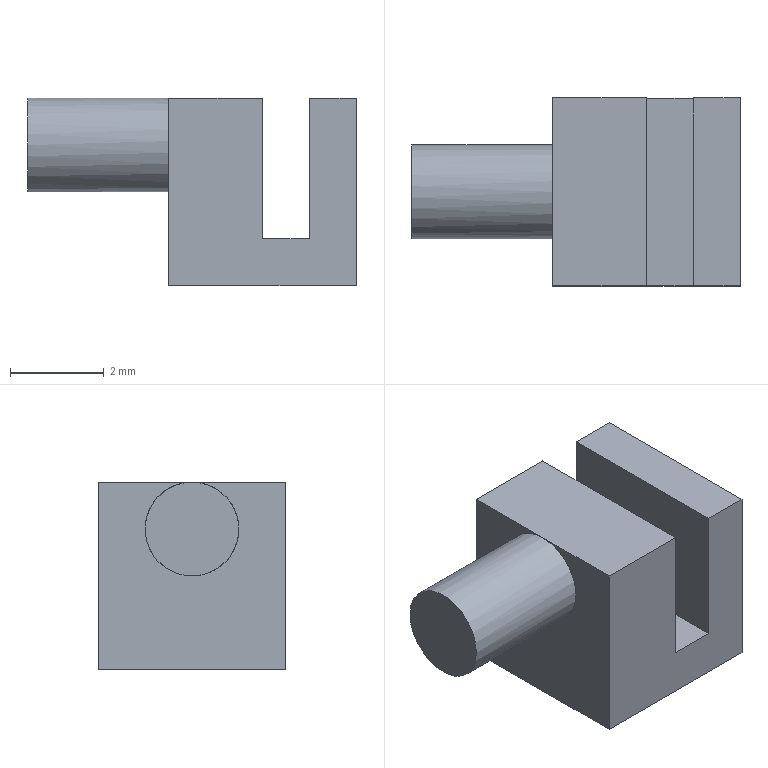Part | STEP file | 1-63.6 | 1 solid | 12 faces | box 7 x 4 x 4 mm | volume 61.425 mm3 | plane 11 | cylinder 1 | commonest cylinder face diameters 2 x1
STEP:
#1=CARTESIAN_POINT('',(0.,0.,0.));
#2=DIRECTION('',(0.,0.,1.));
#3=DIRECTION('',(1.,0.,0.));
#4=AXIS2_PLACEMENT_3D('',#1,#2,#3);
#5=CARTESIAN_POINT('',(-1.5,1.,0.));
#6=VERTEX_POINT('',#5);
#7=CARTESIAN_POINT('',(-1.5,0.,0.));
#8=DIRECTION('',(1.,0.,0.));
#9=DIRECTION('',(0.,1.,0.));
#10=AXIS2_PLACEMENT_3D('',#7,#8,#9);
#11=CIRCLE('',#10,1.);
#12=CARTESIAN_POINT('',(-1.5,-0.2679,0.));
#13=DIRECTION('',(1.,0.,0.));
#14=DIRECTION('',(0.,1.,0.));
#15=AXIS2_PLACEMENT_3D('',#12,#13,#14);
#16=PLANE('',#15);
#17=CARTESIAN_POINT('',(0.2679,0.));
#18=DIRECTION('',(1.,0.));
#19=AXIS2_PLACEMENT_2D('',#17,#18);
#20=CIRCLE('',#19,1.);
#21=(GEOMETRIC_REPRESENTATION_CONTEXT(2)PARAMETRIC_REPRESENTATION_CONTEXT()REPRESENTATION_CONTEXT('',''));
#22=DEFINITIONAL_REPRESENTATION('',(#20),#21);
#23=PCURVE('',#16,#22);
#24=CARTESIAN_POINT('',(1.5,0.,0.));
#25=DIRECTION('',(-1.,0.,0.));
#26=DIRECTION('',(0.,1.,0.));
#27=AXIS2_PLACEMENT_3D('',#24,#25,#26);
#28=CYLINDRICAL_SURFACE('',#27,1.);
#29=CARTESIAN_POINT('',(6.283,3.));
#30=DIRECTION('',(-1.,0.));
#31=VECTOR('',#30,1.);
#32=LINE('',#29,#31);
#33=(GEOMETRIC_REPRESENTATION_CONTEXT(2)PARAMETRIC_REPRESENTATION_CONTEXT()REPRESENTATION_CONTEXT('',''));
#34=DEFINITIONAL_REPRESENTATION('',(#32),#33);
#35=PCURVE('',#28,#34);
#36=SURFACE_CURVE('',#11,(#23,#35),.PCURVE_S1.);
#37=EDGE_CURVE('',#6,#6,#36,.T.);
#38=ORIENTED_EDGE('',*,*,#37,.T.);
#39=EDGE_LOOP('',(#38));
#40=FACE_BOUND('',#39,.F.);
#41=ADVANCED_FACE('',(#40),#16,.F.);
#42=CARTESIAN_POINT('',(1.5,1.,0.));
#43=VERTEX_POINT('',#42);
#44=CARTESIAN_POINT('',(1.5,1.,0.));
#45=DIRECTION('',(-1.,0.,0.));
#46=VECTOR('',#45,1.);
#47=LINE('',#44,#46);
#48=CARTESIAN_POINT('',(6.283,0.));
#49=DIRECTION('',(0.,1.));
#50=VECTOR('',#49,1.);
#51=LINE('',#48,#50);
#52=(GEOMETRIC_REPRESENTATION_CONTEXT(2)PARAMETRIC_REPRESENTATION_CONTEXT()REPRESENTATION_CONTEXT('',''));
#53=DEFINITIONAL_REPRESENTATION('',(#51),#52);
#54=PCURVE('',#28,#53);
#55=CARTESIAN_POINT('',(0.,0.));
#56=DIRECTION('',(0.,1.));
#57=VECTOR('',#56,1.);
#58=LINE('',#55,#57);
#59=(GEOMETRIC_REPRESENTATION_CONTEXT(2)PARAMETRIC_REPRESENTATION_CONTEXT()REPRESENTATION_CONTEXT('',''));
#60=DEFINITIONAL_REPRESENTATION('',(#58),#59);
#61=PCURVE('',#28,#60);
#62=SEAM_CURVE('',#47,(#54,#61),.PCURVE_S1.);
#63=EDGE_CURVE('',#43,#6,#62,.T.);
#64=ORIENTED_EDGE('',*,*,#63,.T.);
#65=ORIENTED_EDGE('',*,*,#37,.T.);
#66=ORIENTED_EDGE('',*,*,#63,.F.);
#67=CARTESIAN_POINT('',(1.5,0.,1.));
#68=VERTEX_POINT('',#67);
#69=CARTESIAN_POINT('',(1.5,0.,0.));
#70=DIRECTION('',(1.,0.,0.));
#71=DIRECTION('',(0.,0.,1.));
#72=AXIS2_PLACEMENT_3D('',#69,#70,#71);
#73=CIRCLE('',#72,1.);
#74=CARTESIAN_POINT('',(4.712,0.));
#75=DIRECTION('',(-1.,0.));
#76=VECTOR('',#75,1.);
#77=LINE('',#74,#76);
#78=(GEOMETRIC_REPRESENTATION_CONTEXT(2)PARAMETRIC_REPRESENTATION_CONTEXT()REPRESENTATION_CONTEXT('',''));
#79=DEFINITIONAL_REPRESENTATION('',(#77),#78);
#80=PCURVE('',#28,#79);
#81=CARTESIAN_POINT('',(1.5,0.,-1.));
#82=DIRECTION('',(1.,0.,0.));
#83=DIRECTION('',(0.,0.,-1.));
#84=AXIS2_PLACEMENT_3D('',#81,#82,#83);
#85=PLANE('',#84);
#86=CARTESIAN_POINT('',(-1.,0.));
#87=DIRECTION('',(-1.,0.));
#88=AXIS2_PLACEMENT_2D('',#86,#87);
#89=CIRCLE('',#88,1.);
#90=(GEOMETRIC_REPRESENTATION_CONTEXT(2)PARAMETRIC_REPRESENTATION_CONTEXT()REPRESENTATION_CONTEXT('',''));
#91=DEFINITIONAL_REPRESENTATION('',(#89),#90);
#92=PCURVE('',#85,#91);
#93=SURFACE_CURVE('',#73,(#80,#92),.PCURVE_S1.);
#94=EDGE_CURVE('',#68,#43,#93,.T.);
#95=ORIENTED_EDGE('',*,*,#94,.F.);
#96=CARTESIAN_POINT('',(1.5,0.,0.));
#97=DIRECTION('',(1.,0.,0.));
#98=DIRECTION('',(0.,1.,0.));
#99=AXIS2_PLACEMENT_3D('',#96,#97,#98);
#100=CIRCLE('',#99,1.);
#101=CARTESIAN_POINT('',(6.283,0.));
#102=DIRECTION('',(-1.,0.));
#103=VECTOR('',#102,1.);
#104=LINE('',#101,#103);
#105=(GEOMETRIC_REPRESENTATION_CONTEXT(2)PARAMETRIC_REPRESENTATION_CONTEXT()REPRESENTATION_CONTEXT('',''));
#106=DEFINITIONAL_REPRESENTATION('',(#104),#105);
#107=PCURVE('',#28,#106);
#108=CARTESIAN_POINT('',(-1.,0.));
#109=DIRECTION('',(0.,1.));
#110=AXIS2_PLACEMENT_2D('',#108,#109);
#111=CIRCLE('',#110,1.);
#112=(GEOMETRIC_REPRESENTATION_CONTEXT(2)PARAMETRIC_REPRESENTATION_CONTEXT()REPRESENTATION_CONTEXT('',''));
#113=DEFINITIONAL_REPRESENTATION('',(#111),#112);
#114=PCURVE('',#85,#113);
#115=SURFACE_CURVE('',#100,(#107,#114),.PCURVE_S1.);
#116=EDGE_CURVE('',#43,#68,#115,.T.);
#117=ORIENTED_EDGE('',*,*,#116,.F.);
#118=EDGE_LOOP('',(#64,#65,#66,#95,#117));
#119=FACE_BOUND('',#118,.T.);
#120=ADVANCED_FACE('',(#119),#28,.T.);
#121=CARTESIAN_POINT('',(1.5,2.,1.));
#122=VERTEX_POINT('',#121);
#123=CARTESIAN_POINT('',(1.5,0.,1.));
#124=VERTEX_POINT('',#123);
#125=CARTESIAN_POINT('',(1.5,2.,1.));
#126=DIRECTION('',(0.,-1.,0.));
#127=VECTOR('',#126,1.);
#128=LINE('',#125,#127);
#129=CARTESIAN_POINT('',(-2.,2.));
#130=DIRECTION('',(0.,-1.));
#131=VECTOR('',#130,1.);
#132=LINE('',#129,#131);
#133=(GEOMETRIC_REPRESENTATION_CONTEXT(2)PARAMETRIC_REPRESENTATION_CONTEXT()REPRESENTATION_CONTEXT('',''));
#134=DEFINITIONAL_REPRESENTATION('',(#132),#133);
#135=PCURVE('',#85,#134);
#136=CARTESIAN_POINT('',(3.5,0.,1.));
#137=DIRECTION('',(0.,0.,1.));
#138=DIRECTION('',(0.,-1.,0.));
#139=AXIS2_PLACEMENT_3D('',#136,#137,#138);
#140=PLANE('',#139);
#141=CARTESIAN_POINT('',(-2.,-2.));
#142=DIRECTION('',(1.,0.));
#143=VECTOR('',#142,1.);
#144=LINE('',#141,#143);
#145=(GEOMETRIC_REPRESENTATION_CONTEXT(2)PARAMETRIC_REPRESENTATION_CONTEXT()REPRESENTATION_CONTEXT('',''));
#146=DEFINITIONAL_REPRESENTATION('',(#144),#145);
#147=PCURVE('',#140,#146);
#148=SURFACE_CURVE('',#128,(#135,#147),.PCURVE_S1.);
#149=EDGE_CURVE('',#122,#124,#148,.T.);
#150=ORIENTED_EDGE('',*,*,#149,.T.);
#151=CARTESIAN_POINT('',(1.5,-2.,1.));
#152=VERTEX_POINT('',#151);
#153=CARTESIAN_POINT('',(1.5,0.,1.));
#154=DIRECTION('',(0.,-1.,0.));
#155=VECTOR('',#154,1.);
#156=LINE('',#153,#155);
#157=CARTESIAN_POINT('',(-2.,0.));
#158=DIRECTION('',(0.,-1.));
#159=VECTOR('',#158,1.);
#160=LINE('',#157,#159);
#161=(GEOMETRIC_REPRESENTATION_CONTEXT(2)PARAMETRIC_REPRESENTATION_CONTEXT()REPRESENTATION_CONTEXT('',''));
#162=DEFINITIONAL_REPRESENTATION('',(#160),#161);
#163=PCURVE('',#85,#162);
#164=CARTESIAN_POINT('',(0.,-2.));
#165=DIRECTION('',(1.,0.));
#166=VECTOR('',#165,1.);
#167=LINE('',#164,#166);
#168=(GEOMETRIC_REPRESENTATION_CONTEXT(2)PARAMETRIC_REPRESENTATION_CONTEXT()REPRESENTATION_CONTEXT('',''));
#169=DEFINITIONAL_REPRESENTATION('',(#167),#168);
#170=PCURVE('',#140,#169);
#171=SURFACE_CURVE('',#156,(#163,#170),.PCURVE_S1.);
#172=EDGE_CURVE('',#124,#152,#171,.T.);
#173=ORIENTED_EDGE('',*,*,#172,.T.);
#174=CARTESIAN_POINT('',(1.5,-2.,-3.));
#175=VERTEX_POINT('',#174);
#176=CARTESIAN_POINT('',(1.5,-2.,1.));
#177=DIRECTION('',(0.,0.,-1.));
#178=VECTOR('',#177,1.);
#179=LINE('',#176,#178);
#180=CARTESIAN_POINT('',(-2.,-2.));
#181=DIRECTION('',(1.,0.));
#182=VECTOR('',#181,1.);
#183=LINE('',#180,#182);
#184=(GEOMETRIC_REPRESENTATION_CONTEXT(2)PARAMETRIC_REPRESENTATION_CONTEXT()REPRESENTATION_CONTEXT('',''));
#185=DEFINITIONAL_REPRESENTATION('',(#183),#184);
#186=PCURVE('',#85,#185);
#187=CARTESIAN_POINT('',(3.5,-2.,-1.));
#188=DIRECTION('',(0.,-1.,0.));
#189=DIRECTION('',(0.,0.,-1.));
#190=AXIS2_PLACEMENT_3D('',#187,#188,#189);
#191=PLANE('',#190);
#192=CARTESIAN_POINT('',(-2.,-2.));
#193=DIRECTION('',(1.,0.));
#194=VECTOR('',#193,1.);
#195=LINE('',#192,#194);
#196=(GEOMETRIC_REPRESENTATION_CONTEXT(2)PARAMETRIC_REPRESENTATION_CONTEXT()REPRESENTATION_CONTEXT('',''));
#197=DEFINITIONAL_REPRESENTATION('',(#195),#196);
#198=PCURVE('',#191,#197);
#199=SURFACE_CURVE('',#179,(#186,#198),.PCURVE_S1.);
#200=EDGE_CURVE('',#152,#175,#199,.T.);
#201=ORIENTED_EDGE('',*,*,#200,.T.);
#202=CARTESIAN_POINT('',(1.5,2.,-3.));
#203=VERTEX_POINT('',#202);
#204=CARTESIAN_POINT('',(1.5,-2.,-3.));
#205=DIRECTION('',(0.,1.,0.));
#206=VECTOR('',#205,1.);
#207=LINE('',#204,#206);
#208=CARTESIAN_POINT('',(2.,-2.));
#209=DIRECTION('',(0.,1.));
#210=VECTOR('',#209,1.);
#211=LINE('',#208,#210);
#212=(GEOMETRIC_REPRESENTATION_CONTEXT(2)PARAMETRIC_REPRESENTATION_CONTEXT()REPRESENTATION_CONTEXT('',''));
#213=DEFINITIONAL_REPRESENTATION('',(#211),#212);
#214=PCURVE('',#85,#213);
#215=CARTESIAN_POINT('',(3.5,0.,-3.));
#216=DIRECTION('',(0.,0.,-1.));
#217=DIRECTION('',(0.,1.,0.));
#218=AXIS2_PLACEMENT_3D('',#215,#216,#217);
#219=PLANE('',#218);
#220=CARTESIAN_POINT('',(-2.,-2.));
#221=DIRECTION('',(1.,0.));
#222=VECTOR('',#221,1.);
#223=LINE('',#220,#222);
#224=(GEOMETRIC_REPRESENTATION_CONTEXT(2)PARAMETRIC_REPRESENTATION_CONTEXT()REPRESENTATION_CONTEXT('',''));
#225=DEFINITIONAL_REPRESENTATION('',(#223),#224);
#226=PCURVE('',#219,#225);
#227=SURFACE_CURVE('',#207,(#214,#226),.PCURVE_S1.);
#228=EDGE_CURVE('',#175,#203,#227,.T.);
#229=ORIENTED_EDGE('',*,*,#228,.T.);
#230=CARTESIAN_POINT('',(1.5,2.,-3.));
#231=DIRECTION('',(0.,0.,1.));
#232=VECTOR('',#231,1.);
#233=LINE('',#230,#232);
#234=CARTESIAN_POINT('',(2.,2.));
#235=DIRECTION('',(-1.,0.));
#236=VECTOR('',#235,1.);
#237=LINE('',#234,#236);
#238=(GEOMETRIC_REPRESENTATION_CONTEXT(2)PARAMETRIC_REPRESENTATION_CONTEXT()REPRESENTATION_CONTEXT('',''));
#239=DEFINITIONAL_REPRESENTATION('',(#237),#238);
#240=PCURVE('',#85,#239);
#241=CARTESIAN_POINT('',(3.5,2.,-1.));
#242=DIRECTION('',(0.,1.,0.));
#243=DIRECTION('',(0.,0.,1.));
#244=AXIS2_PLACEMENT_3D('',#241,#242,#243);
#245=PLANE('',#244);
#246=CARTESIAN_POINT('',(-2.,-2.));
#247=DIRECTION('',(1.,0.));
#248=VECTOR('',#247,1.);
#249=LINE('',#246,#248);
#250=(GEOMETRIC_REPRESENTATION_CONTEXT(2)PARAMETRIC_REPRESENTATION_CONTEXT()REPRESENTATION_CONTEXT('',''));
#251=DEFINITIONAL_REPRESENTATION('',(#249),#250);
#252=PCURVE('',#245,#251);
#253=SURFACE_CURVE('',#233,(#240,#252),.PCURVE_S1.);
#254=EDGE_CURVE('',#203,#122,#253,.T.);
#255=ORIENTED_EDGE('',*,*,#254,.T.);
#256=EDGE_LOOP('',(#150,#173,#201,#229,#255));
#257=FACE_BOUND('',#256,.F.);
#258=ORIENTED_EDGE('',*,*,#116,.F.);
#259=ORIENTED_EDGE('',*,*,#94,.F.);
#260=EDGE_LOOP('',(#258,#259));
#261=FACE_BOUND('',#260,.F.);
#262=ADVANCED_FACE('',(#257,#261),#85,.F.);
#263=ORIENTED_EDGE('',*,*,#228,.T.);
#264=CARTESIAN_POINT('',(5.5,2.,-3.));
#265=VERTEX_POINT('',#264);
#266=CARTESIAN_POINT('',(1.5,2.,-3.));
#267=DIRECTION('',(1.,0.,0.));
#268=VECTOR('',#267,1.);
#269=LINE('',#266,#268);
#270=CARTESIAN_POINT('',(2.,-2.));
#271=DIRECTION('',(0.,1.));
#272=VECTOR('',#271,1.);
#273=LINE('',#270,#272);
#274=(GEOMETRIC_REPRESENTATION_CONTEXT(2)PARAMETRIC_REPRESENTATION_CONTEXT()REPRESENTATION_CONTEXT('',''));
#275=DEFINITIONAL_REPRESENTATION('',(#273),#274);
#276=PCURVE('',#219,#275);
#277=CARTESIAN_POINT('',(-2.,-2.));
#278=DIRECTION('',(0.,1.));
#279=VECTOR('',#278,1.);
#280=LINE('',#277,#279);
#281=(GEOMETRIC_REPRESENTATION_CONTEXT(2)PARAMETRIC_REPRESENTATION_CONTEXT()REPRESENTATION_CONTEXT('',''));
#282=DEFINITIONAL_REPRESENTATION('',(#280),#281);
#283=PCURVE('',#245,#282);
#284=SURFACE_CURVE('',#269,(#276,#283),.PCURVE_S1.);
#285=EDGE_CURVE('',#203,#265,#284,.T.);
#286=ORIENTED_EDGE('',*,*,#285,.T.);
#287=CARTESIAN_POINT('',(5.5,-2.,-3.));
#288=VERTEX_POINT('',#287);
#289=CARTESIAN_POINT('',(5.5,-2.,-3.));
#290=DIRECTION('',(0.,1.,0.));
#291=VECTOR('',#290,1.);
#292=LINE('',#289,#291);
#293=CARTESIAN_POINT('',(-2.,2.));
#294=DIRECTION('',(1.,0.));
#295=VECTOR('',#294,1.);
#296=LINE('',#293,#295);
#297=(GEOMETRIC_REPRESENTATION_CONTEXT(2)PARAMETRIC_REPRESENTATION_CONTEXT()REPRESENTATION_CONTEXT('',''));
#298=DEFINITIONAL_REPRESENTATION('',(#296),#297);
#299=PCURVE('',#219,#298);
#300=CARTESIAN_POINT('',(5.5,0.,-1.));
#301=DIRECTION('',(1.,0.,0.));
#302=DIRECTION('',(0.,0.,-1.));
#303=AXIS2_PLACEMENT_3D('',#300,#301,#302);
#304=PLANE('',#303);
#305=CARTESIAN_POINT('',(2.,-2.));
#306=DIRECTION('',(0.,1.));
#307=VECTOR('',#306,1.);
#308=LINE('',#305,#307);
#309=(GEOMETRIC_REPRESENTATION_CONTEXT(2)PARAMETRIC_REPRESENTATION_CONTEXT()REPRESENTATION_CONTEXT('',''));
#310=DEFINITIONAL_REPRESENTATION('',(#308),#309);
#311=PCURVE('',#304,#310);
#312=SURFACE_CURVE('',#292,(#299,#311),.PCURVE_S1.);
#313=EDGE_CURVE('',#288,#265,#312,.T.);
#314=ORIENTED_EDGE('',*,*,#313,.F.);
#315=CARTESIAN_POINT('',(1.5,-2.,-3.));
#316=DIRECTION('',(1.,0.,0.));
#317=VECTOR('',#316,1.);
#318=LINE('',#315,#317);
#319=CARTESIAN_POINT('',(-2.,-2.));
#320=DIRECTION('',(0.,1.));
#321=VECTOR('',#320,1.);
#322=LINE('',#319,#321);
#323=(GEOMETRIC_REPRESENTATION_CONTEXT(2)PARAMETRIC_REPRESENTATION_CONTEXT()REPRESENTATION_CONTEXT('',''));
#324=DEFINITIONAL_REPRESENTATION('',(#322),#323);
#325=PCURVE('',#219,#324);
#326=CARTESIAN_POINT('',(2.,-2.));
#327=DIRECTION('',(0.,1.));
#328=VECTOR('',#327,1.);
#329=LINE('',#326,#328);
#330=(GEOMETRIC_REPRESENTATION_CONTEXT(2)PARAMETRIC_REPRESENTATION_CONTEXT()REPRESENTATION_CONTEXT('',''));
#331=DEFINITIONAL_REPRESENTATION('',(#329),#330);
#332=PCURVE('',#191,#331);
#333=SURFACE_CURVE('',#318,(#325,#332),.PCURVE_S1.);
#334=EDGE_CURVE('',#175,#288,#333,.T.);
#335=ORIENTED_EDGE('',*,*,#334,.F.);
#336=EDGE_LOOP('',(#263,#286,#314,#335));
#337=FACE_BOUND('',#336,.T.);
#338=ADVANCED_FACE('',(#337),#219,.T.);
#339=CARTESIAN_POINT('',(5.5,-2.,1.));
#340=VERTEX_POINT('',#339);
#341=CARTESIAN_POINT('',(5.5,-2.,1.));
#342=DIRECTION('',(0.,0.,-1.));
#343=VECTOR('',#342,1.);
#344=LINE('',#341,#343);
#345=CARTESIAN_POINT('',(-2.,-2.));
#346=DIRECTION('',(1.,0.));
#347=VECTOR('',#346,1.);
#348=LINE('',#345,#347);
#349=(GEOMETRIC_REPRESENTATION_CONTEXT(2)PARAMETRIC_REPRESENTATION_CONTEXT()REPRESENTATION_CONTEXT('',''));
#350=DEFINITIONAL_REPRESENTATION('',(#348),#349);
#351=PCURVE('',#304,#350);
#352=CARTESIAN_POINT('',(-2.,2.));
#353=DIRECTION('',(1.,0.));
#354=VECTOR('',#353,1.);
#355=LINE('',#352,#354);
#356=(GEOMETRIC_REPRESENTATION_CONTEXT(2)PARAMETRIC_REPRESENTATION_CONTEXT()REPRESENTATION_CONTEXT('',''));
#357=DEFINITIONAL_REPRESENTATION('',(#355),#356);
#358=PCURVE('',#191,#357);
#359=SURFACE_CURVE('',#344,(#351,#358),.PCURVE_S1.);
#360=EDGE_CURVE('',#340,#288,#359,.T.);
#361=ORIENTED_EDGE('',*,*,#360,.T.);
#362=ORIENTED_EDGE('',*,*,#313,.T.);
#363=CARTESIAN_POINT('',(5.5,2.,1.));
#364=VERTEX_POINT('',#363);
#365=CARTESIAN_POINT('',(5.5,2.,-3.));
#366=DIRECTION('',(0.,0.,1.));
#367=VECTOR('',#366,1.);
#368=LINE('',#365,#367);
#369=CARTESIAN_POINT('',(2.,2.));
#370=DIRECTION('',(-1.,0.));
#371=VECTOR('',#370,1.);
#372=LINE('',#369,#371);
#373=(GEOMETRIC_REPRESENTATION_CONTEXT(2)PARAMETRIC_REPRESENTATION_CONTEXT()REPRESENTATION_CONTEXT('',''));
#374=DEFINITIONAL_REPRESENTATION('',(#372),#373);
#375=PCURVE('',#304,#374);
#376=CARTESIAN_POINT('',(-2.,2.));
#377=DIRECTION('',(1.,0.));
#378=VECTOR('',#377,1.);
#379=LINE('',#376,#378);
#380=(GEOMETRIC_REPRESENTATION_CONTEXT(2)PARAMETRIC_REPRESENTATION_CONTEXT()REPRESENTATION_CONTEXT('',''));
#381=DEFINITIONAL_REPRESENTATION('',(#379),#380);
#382=PCURVE('',#245,#381);
#383=SURFACE_CURVE('',#368,(#375,#382),.PCURVE_S1.);
#384=EDGE_CURVE('',#265,#364,#383,.T.);
#385=ORIENTED_EDGE('',*,*,#384,.T.);
#386=CARTESIAN_POINT('',(5.5,2.,1.));
#387=DIRECTION('',(0.,-1.,0.));
#388=VECTOR('',#387,1.);
#389=LINE('',#386,#388);
#390=CARTESIAN_POINT('',(-2.,2.));
#391=DIRECTION('',(0.,-1.));
#392=VECTOR('',#391,1.);
#393=LINE('',#390,#392);
#394=(GEOMETRIC_REPRESENTATION_CONTEXT(2)PARAMETRIC_REPRESENTATION_CONTEXT()REPRESENTATION_CONTEXT('',''));
#395=DEFINITIONAL_REPRESENTATION('',(#393),#394);
#396=PCURVE('',#304,#395);
#397=CARTESIAN_POINT('',(3.5,0.,1.));
#398=DIRECTION('',(0.,0.,1.));
#399=DIRECTION('',(0.,-1.,0.));
#400=AXIS2_PLACEMENT_3D('',#397,#398,#399);
#401=PLANE('',#400);
#402=CARTESIAN_POINT('',(-2.,2.));
#403=DIRECTION('',(1.,0.));
#404=VECTOR('',#403,1.);
#405=LINE('',#402,#404);
#406=(GEOMETRIC_REPRESENTATION_CONTEXT(2)PARAMETRIC_REPRESENTATION_CONTEXT()REPRESENTATION_CONTEXT('',''));
#407=DEFINITIONAL_REPRESENTATION('',(#405),#406);
#408=PCURVE('',#401,#407);
#409=SURFACE_CURVE('',#389,(#396,#408),.PCURVE_S1.);
#410=EDGE_CURVE('',#364,#340,#409,.T.);
#411=ORIENTED_EDGE('',*,*,#410,.T.);
#412=EDGE_LOOP('',(#361,#362,#385,#411));
#413=FACE_BOUND('',#412,.T.);
#414=ADVANCED_FACE('',(#413),#304,.T.);
#415=ORIENTED_EDGE('',*,*,#200,.T.);
#416=ORIENTED_EDGE('',*,*,#334,.T.);
#417=ORIENTED_EDGE('',*,*,#360,.F.);
#418=CARTESIAN_POINT('',(4.5,-2.,1.));
#419=VERTEX_POINT('',#418);
#420=CARTESIAN_POINT('',(4.5,-2.,1.));
#421=DIRECTION('',(1.,0.,0.));
#422=VECTOR('',#421,1.);
#423=LINE('',#420,#422);
#424=CARTESIAN_POINT('',(-2.,1.));
#425=DIRECTION('',(0.,1.));
#426=VECTOR('',#425,1.);
#427=LINE('',#424,#426);
#428=(GEOMETRIC_REPRESENTATION_CONTEXT(2)PARAMETRIC_REPRESENTATION_CONTEXT()REPRESENTATION_CONTEXT('',''));
#429=DEFINITIONAL_REPRESENTATION('',(#427),#428);
#430=PCURVE('',#191,#429);
#431=CARTESIAN_POINT('',(2.,1.));
#432=DIRECTION('',(0.,1.));
#433=VECTOR('',#432,1.);
#434=LINE('',#431,#433);
#435=(GEOMETRIC_REPRESENTATION_CONTEXT(2)PARAMETRIC_REPRESENTATION_CONTEXT()REPRESENTATION_CONTEXT('',''));
#436=DEFINITIONAL_REPRESENTATION('',(#434),#435);
#437=PCURVE('',#401,#436);
#438=SURFACE_CURVE('',#423,(#430,#437),.PCURVE_S1.);
#439=EDGE_CURVE('',#419,#340,#438,.T.);
#440=ORIENTED_EDGE('',*,*,#439,.F.);
#441=CARTESIAN_POINT('',(4.5,-2.,-2.));
#442=VERTEX_POINT('',#441);
#443=CARTESIAN_POINT('',(4.5,-2.,-2.));
#444=DIRECTION('',(0.,0.,1.));
#445=VECTOR('',#444,1.);
#446=LINE('',#443,#445);
#447=CARTESIAN_POINT('',(1.,1.));
#448=DIRECTION('',(-1.,0.));
#449=VECTOR('',#448,1.);
#450=LINE('',#447,#449);
#451=(GEOMETRIC_REPRESENTATION_CONTEXT(2)PARAMETRIC_REPRESENTATION_CONTEXT()REPRESENTATION_CONTEXT('',''));
#452=DEFINITIONAL_REPRESENTATION('',(#450),#451);
#453=PCURVE('',#191,#452);
#454=CARTESIAN_POINT('',(4.5,0.,0.));
#455=DIRECTION('',(-1.,0.,0.));
#456=DIRECTION('',(0.,0.,1.));
#457=AXIS2_PLACEMENT_3D('',#454,#455,#456);
#458=PLANE('',#457);
#459=CARTESIAN_POINT('',(-2.,-2.));
#460=DIRECTION('',(1.,0.));
#461=VECTOR('',#460,1.);
#462=LINE('',#459,#461);
#463=(GEOMETRIC_REPRESENTATION_CONTEXT(2)PARAMETRIC_REPRESENTATION_CONTEXT()REPRESENTATION_CONTEXT('',''));
#464=DEFINITIONAL_REPRESENTATION('',(#462),#463);
#465=PCURVE('',#458,#464);
#466=SURFACE_CURVE('',#446,(#453,#465),.PCURVE_S1.);
#467=EDGE_CURVE('',#442,#419,#466,.T.);
#468=ORIENTED_EDGE('',*,*,#467,.F.);
#469=CARTESIAN_POINT('',(3.5,-2.,-2.));
#470=VERTEX_POINT('',#469);
#471=CARTESIAN_POINT('',(3.5,-2.,-2.));
#472=DIRECTION('',(1.,0.,0.));
#473=VECTOR('',#472,1.);
#474=LINE('',#471,#473);
#475=CARTESIAN_POINT('',(1.,0.));
#476=DIRECTION('',(0.,1.));
#477=VECTOR('',#476,1.);
#478=LINE('',#475,#477);
#479=(GEOMETRIC_REPRESENTATION_CONTEXT(2)PARAMETRIC_REPRESENTATION_CONTEXT()REPRESENTATION_CONTEXT('',''));
#480=DEFINITIONAL_REPRESENTATION('',(#478),#479);
#481=PCURVE('',#191,#480);
#482=CARTESIAN_POINT('',(4.,0.,-2.));
#483=DIRECTION('',(0.,0.,1.));
#484=DIRECTION('',(0.,-1.,0.));
#485=AXIS2_PLACEMENT_3D('',#482,#483,#484);
#486=PLANE('',#485);
#487=CARTESIAN_POINT('',(2.,-0.5));
#488=DIRECTION('',(0.,1.));
#489=VECTOR('',#488,1.);
#490=LINE('',#487,#489);
#491=(GEOMETRIC_REPRESENTATION_CONTEXT(2)PARAMETRIC_REPRESENTATION_CONTEXT()REPRESENTATION_CONTEXT('',''));
#492=DEFINITIONAL_REPRESENTATION('',(#490),#491);
#493=PCURVE('',#486,#492);
#494=SURFACE_CURVE('',#474,(#481,#493),.PCURVE_S1.);
#495=EDGE_CURVE('',#470,#442,#494,.T.);
#496=ORIENTED_EDGE('',*,*,#495,.F.);
#497=CARTESIAN_POINT('',(3.5,-2.,1.));
#498=VERTEX_POINT('',#497);
#499=CARTESIAN_POINT('',(3.5,-2.,-2.));
#500=DIRECTION('',(0.,0.,1.));
#501=VECTOR('',#500,1.);
#502=LINE('',#499,#501);
#503=CARTESIAN_POINT('',(1.,0.));
#504=DIRECTION('',(-1.,0.));
#505=VECTOR('',#504,1.);
#506=LINE('',#503,#505);
#507=(GEOMETRIC_REPRESENTATION_CONTEXT(2)PARAMETRIC_REPRESENTATION_CONTEXT()REPRESENTATION_CONTEXT('',''));
#508=DEFINITIONAL_REPRESENTATION('',(#506),#507);
#509=PCURVE('',#191,#508);
#510=CARTESIAN_POINT('',(3.5,0.,0.));
#511=DIRECTION('',(-1.,0.,0.));
#512=DIRECTION('',(0.,0.,1.));
#513=AXIS2_PLACEMENT_3D('',#510,#511,#512);
#514=PLANE('',#513);
#515=CARTESIAN_POINT('',(-2.,-2.));
#516=DIRECTION('',(1.,0.));
#517=VECTOR('',#516,1.);
#518=LINE('',#515,#517);
#519=(GEOMETRIC_REPRESENTATION_CONTEXT(2)PARAMETRIC_REPRESENTATION_CONTEXT()REPRESENTATION_CONTEXT('',''));
#520=DEFINITIONAL_REPRESENTATION('',(#518),#519);
#521=PCURVE('',#514,#520);
#522=SURFACE_CURVE('',#502,(#509,#521),.PCURVE_S1.);
#523=EDGE_CURVE('',#470,#498,#522,.T.);
#524=ORIENTED_EDGE('',*,*,#523,.T.);
#525=CARTESIAN_POINT('',(1.5,-2.,1.));
#526=DIRECTION('',(1.,0.,0.));
#527=VECTOR('',#526,1.);
#528=LINE('',#525,#527);
#529=CARTESIAN_POINT('',(-2.,-2.));
#530=DIRECTION('',(0.,1.));
#531=VECTOR('',#530,1.);
#532=LINE('',#529,#531);
#533=(GEOMETRIC_REPRESENTATION_CONTEXT(2)PARAMETRIC_REPRESENTATION_CONTEXT()REPRESENTATION_CONTEXT('',''));
#534=DEFINITIONAL_REPRESENTATION('',(#532),#533);
#535=PCURVE('',#191,#534);
#536=CARTESIAN_POINT('',(2.,-2.));
#537=DIRECTION('',(0.,1.));
#538=VECTOR('',#537,1.);
#539=LINE('',#536,#538);
#540=(GEOMETRIC_REPRESENTATION_CONTEXT(2)PARAMETRIC_REPRESENTATION_CONTEXT()REPRESENTATION_CONTEXT('',''));
#541=DEFINITIONAL_REPRESENTATION('',(#539),#540);
#542=PCURVE('',#140,#541);
#543=SURFACE_CURVE('',#528,(#535,#542),.PCURVE_S1.);
#544=EDGE_CURVE('',#152,#498,#543,.T.);
#545=ORIENTED_EDGE('',*,*,#544,.F.);
#546=EDGE_LOOP('',(#415,#416,#417,#440,#468,#496,#524,#545));
#547=FACE_BOUND('',#546,.T.);
#548=ADVANCED_FACE('',(#547),#191,.T.);
#549=ORIENTED_EDGE('',*,*,#254,.T.);
#550=CARTESIAN_POINT('',(3.5,2.,1.));
#551=VERTEX_POINT('',#550);
#552=CARTESIAN_POINT('',(1.5,2.,1.));
#553=DIRECTION('',(1.,0.,0.));
#554=VECTOR('',#553,1.);
#555=LINE('',#552,#554);
#556=CARTESIAN_POINT('',(2.,-2.));
#557=DIRECTION('',(0.,1.));
#558=VECTOR('',#557,1.);
#559=LINE('',#556,#558);
#560=(GEOMETRIC_REPRESENTATION_CONTEXT(2)PARAMETRIC_REPRESENTATION_CONTEXT()REPRESENTATION_CONTEXT('',''));
#561=DEFINITIONAL_REPRESENTATION('',(#559),#560);
#562=PCURVE('',#245,#561);
#563=CARTESIAN_POINT('',(-2.,-2.));
#564=DIRECTION('',(0.,1.));
#565=VECTOR('',#564,1.);
#566=LINE('',#563,#565);
#567=(GEOMETRIC_REPRESENTATION_CONTEXT(2)PARAMETRIC_REPRESENTATION_CONTEXT()REPRESENTATION_CONTEXT('',''));
#568=DEFINITIONAL_REPRESENTATION('',(#566),#567);
#569=PCURVE('',#140,#568);
#570=SURFACE_CURVE('',#555,(#562,#569),.PCURVE_S1.);
#571=EDGE_CURVE('',#122,#551,#570,.T.);
#572=ORIENTED_EDGE('',*,*,#571,.T.);
#573=CARTESIAN_POINT('',(3.5,2.,-2.));
#574=VERTEX_POINT('',#573);
#575=CARTESIAN_POINT('',(3.5,2.,1.));
#576=DIRECTION('',(0.,0.,-1.));
#577=VECTOR('',#576,1.);
#578=LINE('',#575,#577);
#579=CARTESIAN_POINT('',(2.,0.));
#580=DIRECTION('',(-1.,0.));
#581=VECTOR('',#580,1.);
#582=LINE('',#579,#581);
#583=(GEOMETRIC_REPRESENTATION_CONTEXT(2)PARAMETRIC_REPRESENTATION_CONTEXT()REPRESENTATION_CONTEXT('',''));
#584=DEFINITIONAL_REPRESENTATION('',(#582),#583);
#585=PCURVE('',#245,#584);
#586=CARTESIAN_POINT('',(1.,2.));
#587=DIRECTION('',(-1.,0.));
#588=VECTOR('',#587,1.);
#589=LINE('',#586,#588);
#590=(GEOMETRIC_REPRESENTATION_CONTEXT(2)PARAMETRIC_REPRESENTATION_CONTEXT()REPRESENTATION_CONTEXT('',''));
#591=DEFINITIONAL_REPRESENTATION('',(#589),#590);
#592=PCURVE('',#514,#591);
#593=SURFACE_CURVE('',#578,(#585,#592),.PCURVE_S1.);
#594=EDGE_CURVE('',#551,#574,#593,.T.);
#595=ORIENTED_EDGE('',*,*,#594,.T.);
#596=CARTESIAN_POINT('',(4.5,2.,-2.));
#597=VERTEX_POINT('',#596);
#598=CARTESIAN_POINT('',(3.5,2.,-2.));
#599=DIRECTION('',(1.,0.,0.));
#600=VECTOR('',#599,1.);
#601=LINE('',#598,#600);
#602=CARTESIAN_POINT('',(-1.,0.));
#603=DIRECTION('',(0.,1.));
#604=VECTOR('',#603,1.);
#605=LINE('',#602,#604);
#606=(GEOMETRIC_REPRESENTATION_CONTEXT(2)PARAMETRIC_REPRESENTATION_CONTEXT()REPRESENTATION_CONTEXT('',''));
#607=DEFINITIONAL_REPRESENTATION('',(#605),#606);
#608=PCURVE('',#245,#607);
#609=CARTESIAN_POINT('',(-2.,-0.5));
#610=DIRECTION('',(0.,1.));
#611=VECTOR('',#610,1.);
#612=LINE('',#609,#611);
#613=(GEOMETRIC_REPRESENTATION_CONTEXT(2)PARAMETRIC_REPRESENTATION_CONTEXT()REPRESENTATION_CONTEXT('',''));
#614=DEFINITIONAL_REPRESENTATION('',(#612),#613);
#615=PCURVE('',#486,#614);
#616=SURFACE_CURVE('',#601,(#608,#615),.PCURVE_S1.);
#617=EDGE_CURVE('',#574,#597,#616,.T.);
#618=ORIENTED_EDGE('',*,*,#617,.T.);
#619=CARTESIAN_POINT('',(4.5,2.,1.));
#620=VERTEX_POINT('',#619);
#621=CARTESIAN_POINT('',(4.5,2.,1.));
#622=DIRECTION('',(0.,0.,-1.));
#623=VECTOR('',#622,1.);
#624=LINE('',#621,#623);
#625=CARTESIAN_POINT('',(2.,1.));
#626=DIRECTION('',(-1.,0.));
#627=VECTOR('',#626,1.);
#628=LINE('',#625,#627);
#629=(GEOMETRIC_REPRESENTATION_CONTEXT(2)PARAMETRIC_REPRESENTATION_CONTEXT()REPRESENTATION_CONTEXT('',''));
#630=DEFINITIONAL_REPRESENTATION('',(#628),#629);
#631=PCURVE('',#245,#630);
#632=CARTESIAN_POINT('',(1.,2.));
#633=DIRECTION('',(-1.,0.));
#634=VECTOR('',#633,1.);
#635=LINE('',#632,#634);
#636=(GEOMETRIC_REPRESENTATION_CONTEXT(2)PARAMETRIC_REPRESENTATION_CONTEXT()REPRESENTATION_CONTEXT('',''));
#637=DEFINITIONAL_REPRESENTATION('',(#635),#636);
#638=PCURVE('',#458,#637);
#639=SURFACE_CURVE('',#624,(#631,#638),.PCURVE_S1.);
#640=EDGE_CURVE('',#620,#597,#639,.T.);
#641=ORIENTED_EDGE('',*,*,#640,.F.);
#642=CARTESIAN_POINT('',(4.5,2.,1.));
#643=DIRECTION('',(1.,0.,0.));
#644=VECTOR('',#643,1.);
#645=LINE('',#642,#644);
#646=CARTESIAN_POINT('',(2.,1.));
#647=DIRECTION('',(0.,1.));
#648=VECTOR('',#647,1.);
#649=LINE('',#646,#648);
#650=(GEOMETRIC_REPRESENTATION_CONTEXT(2)PARAMETRIC_REPRESENTATION_CONTEXT()REPRESENTATION_CONTEXT('',''));
#651=DEFINITIONAL_REPRESENTATION('',(#649),#650);
#652=PCURVE('',#245,#651);
#653=CARTESIAN_POINT('',(-2.,1.));
#654=DIRECTION('',(0.,1.));
#655=VECTOR('',#654,1.);
#656=LINE('',#653,#655);
#657=(GEOMETRIC_REPRESENTATION_CONTEXT(2)PARAMETRIC_REPRESENTATION_CONTEXT()REPRESENTATION_CONTEXT('',''));
#658=DEFINITIONAL_REPRESENTATION('',(#656),#657);
#659=PCURVE('',#401,#658);
#660=SURFACE_CURVE('',#645,(#652,#659),.PCURVE_S1.);
#661=EDGE_CURVE('',#620,#364,#660,.T.);
#662=ORIENTED_EDGE('',*,*,#661,.T.);
#663=ORIENTED_EDGE('',*,*,#384,.F.);
#664=ORIENTED_EDGE('',*,*,#285,.F.);
#665=EDGE_LOOP('',(#549,#572,#595,#618,#641,#662,#663,#664));
#666=FACE_BOUND('',#665,.T.);
#667=ADVANCED_FACE('',(#666),#245,.T.);
#668=ORIENTED_EDGE('',*,*,#149,.T.);
#669=ORIENTED_EDGE('',*,*,#172,.T.);
#670=ORIENTED_EDGE('',*,*,#544,.T.);
#671=CARTESIAN_POINT('',(3.5,-2.,1.));
#672=DIRECTION('',(0.,1.,0.));
#673=VECTOR('',#672,1.);
#674=LINE('',#671,#673);
#675=CARTESIAN_POINT('',(2.,0.));
#676=DIRECTION('',(-1.,0.));
#677=VECTOR('',#676,1.);
#678=LINE('',#675,#677);
#679=(GEOMETRIC_REPRESENTATION_CONTEXT(2)PARAMETRIC_REPRESENTATION_CONTEXT()REPRESENTATION_CONTEXT('',''));
#680=DEFINITIONAL_REPRESENTATION('',(#678),#679);
#681=PCURVE('',#140,#680);
#682=CARTESIAN_POINT('',(1.,-2.));
#683=DIRECTION('',(0.,1.));
#684=VECTOR('',#683,1.);
#685=LINE('',#682,#684);
#686=(GEOMETRIC_REPRESENTATION_CONTEXT(2)PARAMETRIC_REPRESENTATION_CONTEXT()REPRESENTATION_CONTEXT('',''));
#687=DEFINITIONAL_REPRESENTATION('',(#685),#686);
#688=PCURVE('',#514,#687);
#689=SURFACE_CURVE('',#674,(#681,#688),.PCURVE_S1.);
#690=EDGE_CURVE('',#498,#551,#689,.T.);
#691=ORIENTED_EDGE('',*,*,#690,.T.);
#692=ORIENTED_EDGE('',*,*,#571,.F.);
#693=EDGE_LOOP('',(#668,#669,#670,#691,#692));
#694=FACE_BOUND('',#693,.T.);
#695=ADVANCED_FACE('',(#694),#140,.T.);
#696=ORIENTED_EDGE('',*,*,#410,.F.);
#697=ORIENTED_EDGE('',*,*,#661,.F.);
#698=CARTESIAN_POINT('',(4.5,-2.,1.));
#699=DIRECTION('',(0.,1.,0.));
#700=VECTOR('',#699,1.);
#701=LINE('',#698,#700);
#702=CARTESIAN_POINT('',(2.,1.));
#703=DIRECTION('',(-1.,0.));
#704=VECTOR('',#703,1.);
#705=LINE('',#702,#704);
#706=(GEOMETRIC_REPRESENTATION_CONTEXT(2)PARAMETRIC_REPRESENTATION_CONTEXT()REPRESENTATION_CONTEXT('',''));
#707=DEFINITIONAL_REPRESENTATION('',(#705),#706);
#708=PCURVE('',#401,#707);
#709=CARTESIAN_POINT('',(1.,-2.));
#710=DIRECTION('',(0.,1.));
#711=VECTOR('',#710,1.);
#712=LINE('',#709,#711);
#713=(GEOMETRIC_REPRESENTATION_CONTEXT(2)PARAMETRIC_REPRESENTATION_CONTEXT()REPRESENTATION_CONTEXT('',''));
#714=DEFINITIONAL_REPRESENTATION('',(#712),#713);
#715=PCURVE('',#458,#714);
#716=SURFACE_CURVE('',#701,(#708,#715),.PCURVE_S1.);
#717=EDGE_CURVE('',#419,#620,#716,.T.);
#718=ORIENTED_EDGE('',*,*,#717,.F.);
#719=ORIENTED_EDGE('',*,*,#439,.T.);
#720=EDGE_LOOP('',(#696,#697,#718,#719));
#721=FACE_BOUND('',#720,.T.);
#722=ADVANCED_FACE('',(#721),#401,.T.);
#723=ORIENTED_EDGE('',*,*,#467,.T.);
#724=ORIENTED_EDGE('',*,*,#717,.T.);
#725=ORIENTED_EDGE('',*,*,#640,.T.);
#726=CARTESIAN_POINT('',(4.5,2.,-2.));
#727=DIRECTION('',(0.,-1.,0.));
#728=VECTOR('',#727,1.);
#729=LINE('',#726,#728);
#730=CARTESIAN_POINT('',(-2.,2.));
#731=DIRECTION('',(0.,-1.));
#732=VECTOR('',#731,1.);
#733=LINE('',#730,#732);
#734=(GEOMETRIC_REPRESENTATION_CONTEXT(2)PARAMETRIC_REPRESENTATION_CONTEXT()REPRESENTATION_CONTEXT('',''));
#735=DEFINITIONAL_REPRESENTATION('',(#733),#734);
#736=PCURVE('',#458,#735);
#737=CARTESIAN_POINT('',(-2.,0.5));
#738=DIRECTION('',(1.,0.));
#739=VECTOR('',#738,1.);
#740=LINE('',#737,#739);
#741=(GEOMETRIC_REPRESENTATION_CONTEXT(2)PARAMETRIC_REPRESENTATION_CONTEXT()REPRESENTATION_CONTEXT('',''));
#742=DEFINITIONAL_REPRESENTATION('',(#740),#741);
#743=PCURVE('',#486,#742);
#744=SURFACE_CURVE('',#729,(#736,#743),.PCURVE_S1.);
#745=EDGE_CURVE('',#597,#442,#744,.T.);
#746=ORIENTED_EDGE('',*,*,#745,.T.);
#747=EDGE_LOOP('',(#723,#724,#725,#746));
#748=FACE_BOUND('',#747,.T.);
#749=ADVANCED_FACE('',(#748),#458,.T.);
#750=CARTESIAN_POINT('',(3.5,2.,-2.));
#751=DIRECTION('',(0.,-1.,0.));
#752=VECTOR('',#751,1.);
#753=LINE('',#750,#752);
#754=CARTESIAN_POINT('',(-2.,-0.5));
#755=DIRECTION('',(1.,0.));
#756=VECTOR('',#755,1.);
#757=LINE('',#754,#756);
#758=(GEOMETRIC_REPRESENTATION_CONTEXT(2)PARAMETRIC_REPRESENTATION_CONTEXT()REPRESENTATION_CONTEXT('',''));
#759=DEFINITIONAL_REPRESENTATION('',(#757),#758);
#760=PCURVE('',#486,#759);
#761=CARTESIAN_POINT('',(-2.,2.));
#762=DIRECTION('',(0.,-1.));
#763=VECTOR('',#762,1.);
#764=LINE('',#761,#763);
#765=(GEOMETRIC_REPRESENTATION_CONTEXT(2)PARAMETRIC_REPRESENTATION_CONTEXT()REPRESENTATION_CONTEXT('',''));
#766=DEFINITIONAL_REPRESENTATION('',(#764),#765);
#767=PCURVE('',#514,#766);
#768=SURFACE_CURVE('',#753,(#760,#767),.PCURVE_S1.);
#769=EDGE_CURVE('',#574,#470,#768,.T.);
#770=ORIENTED_EDGE('',*,*,#769,.T.);
#771=ORIENTED_EDGE('',*,*,#495,.T.);
#772=ORIENTED_EDGE('',*,*,#745,.F.);
#773=ORIENTED_EDGE('',*,*,#617,.F.);
#774=EDGE_LOOP('',(#770,#771,#772,#773));
#775=FACE_BOUND('',#774,.T.);
#776=ADVANCED_FACE('',(#775),#486,.T.);
#777=ORIENTED_EDGE('',*,*,#523,.T.);
#778=ORIENTED_EDGE('',*,*,#690,.T.);
#779=ORIENTED_EDGE('',*,*,#594,.T.);
#780=ORIENTED_EDGE('',*,*,#769,.T.);
#781=EDGE_LOOP('',(#777,#778,#779,#780));
#782=FACE_BOUND('',#781,.F.);
#783=ADVANCED_FACE('',(#782),#514,.F.);
#784=CLOSED_SHELL('',(#41,#120,#262,#338,#414,#548,#667,#695,#722,#749,#776,#783));
#785=MANIFOLD_SOLID_BREP('',#784);
#786=(LENGTH_UNIT()NAMED_UNIT(*)SI_UNIT(.MILLI.,.METRE.));
#787=UNCERTAINTY_MEASURE_WITH_UNIT(LENGTH_MEASURE(0.0000001),#786,'','');
#788=(NAMED_UNIT(*)PLANE_ANGLE_UNIT()SI_UNIT($,.RADIAN.));
#789=(NAMED_UNIT(*)SI_UNIT($,.STERADIAN.)SOLID_ANGLE_UNIT());
#790=(GEOMETRIC_REPRESENTATION_CONTEXT(3)GLOBAL_UNCERTAINTY_ASSIGNED_CONTEXT((#787))GLOBAL_UNIT_ASSIGNED_CONTEXT((#786,#788,#789))REPRESENTATION_CONTEXT('',''));
#791=ADVANCED_BREP_SHAPE_REPRESENTATION('',(#4,#785),#790);